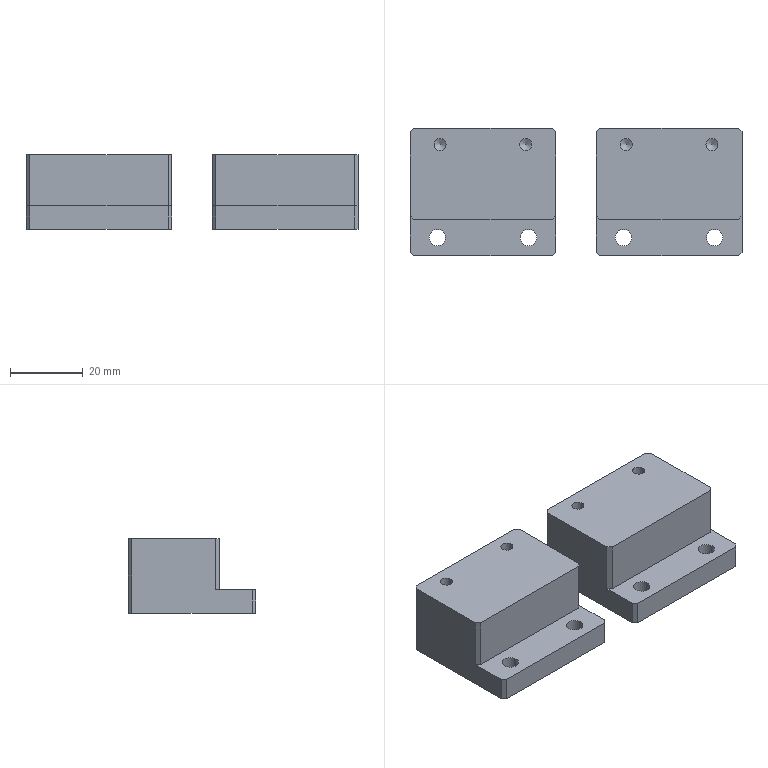CAM job | NX | 3-axis milling, drilling | part box 91 x 35 x 20.5 mm | stock box 96 x 40 x 25 mm
Tools:
number,name,description,diameter,corner_radius,flute_length,length,flutes
9,D10,平底铣刀-粗,10.0,0.0,35.0,75.0,2
7,D6-J,平底铣刀-精,6.0,0.0,25.0,75.0,2
10,D10-J,平底铣刀-精,10.0,0.0,35.0,75.0,2
1,D80R0.8飞刀,圆鼻刀-粗,80.0,0.8,50.0,75.0,2
2,D6倒角刀,倒角刀,6.0,0.0,3.0,25.0,2
21,M4X0.7,丝锥,3.3,0.0,35.0,50.0,2
11,ZT4.5,钻头,4.5,0.0,35.0,50.0,2
13,钻头3.3,Twist Drill 3.3 mm,3.3,0.0,35.0,35.008,2
Operations:
program,operation,operation_type,tool,method,geometry_group,spindle_rpm,surface_speed,feed_per_tooth,feed_cut,feed_plunge,cut_length_mm,path_length_mm,cut_time_min,machine_time_min
A,顶面,FaceMilling,D80R0.8飞刀,侧刃精光-切深K-步距G,W-A,4000.0,1005.31,0.125,1000.0,100.0,185.0,221.0,0.185,0.1886
A,外形粗_2,VolumeBased25DMillingOperation,D10,METHOD,W-A,8000.0,251.327,0.3125,5000.0,80.0,10066.355,10235.455,2.013,2.03
A,底壁铣分层开粗-中_COPY,VolumeBased25DMillingOperation,D10,分层开粗-切深K-步距G,W-A,8000.0,251.327,0.3125,5000.0,100.0,5563.643,5880.409,1.113,1.144
A,打点-深0.8,Operation,D6倒角刀,NONE,W-A,8000.0,150.796,0.0312,500.0,90.0,14.4,269.052,0.0288,0.0543
A,通孔-5-6,Operation,ZT4.5,NONE,W-A,3000.0,42.411,0.025,150.0,90.0,43.408,233.875,0.2894,0.3084
A,盲锥孔-M4螺纹底孔,Operation,钻头3.3,NONE,W-A,3000.0,31.102,0.02,120.0,90.0,53.966,225.492,0.4497,0.4669
A,仅选体,SurfaceContour,D6倒角刀,METHOD,W-A,8000.0,150.796,0.1875,3000.0,100.0,477.953,683.05,0.1593,0.1798
A,钻倒角_1,Operation,D6倒角刀,METHOD,W-A,8000.0,150.796,0.0312,500.0,0.0,20.8,165.645,0.0416,0.0561
A,铣倒角_1,PlanarMilling,D6倒角刀,METHOD,W-A,8000.0,150.796,0.0312,500.0,100.0,69.412,421.483,0.1388,0.174
A,盲锥孔-攻牙M4,Operation,M4X0.7,METHOD,W-A,800.0,8.294,0.0004,0.7,90.0,42.0,201.561,60.0,60.016
A,底精_1,VolumeBased25DMillingOperation,D6-J,METHOD,W-A,6000.0,113.0,0.2083,1200.0,100.0,378.352,563.852,0.3153,0.3338
A,底侧精_3,VolumeBased25DMillingOperation,D6-J,METHOD,W-A,6000.0,113.0,0.2083,1200.0,100.0,206.498,545.659,0.1721,0.206
A,外形半精_2,VolumeBased25DMillingOperation,D10-J,METHOD,W-A,8000.0,251.327,0.0625,1000.0,100.0,736.291,1224.604,0.7363,0.7851